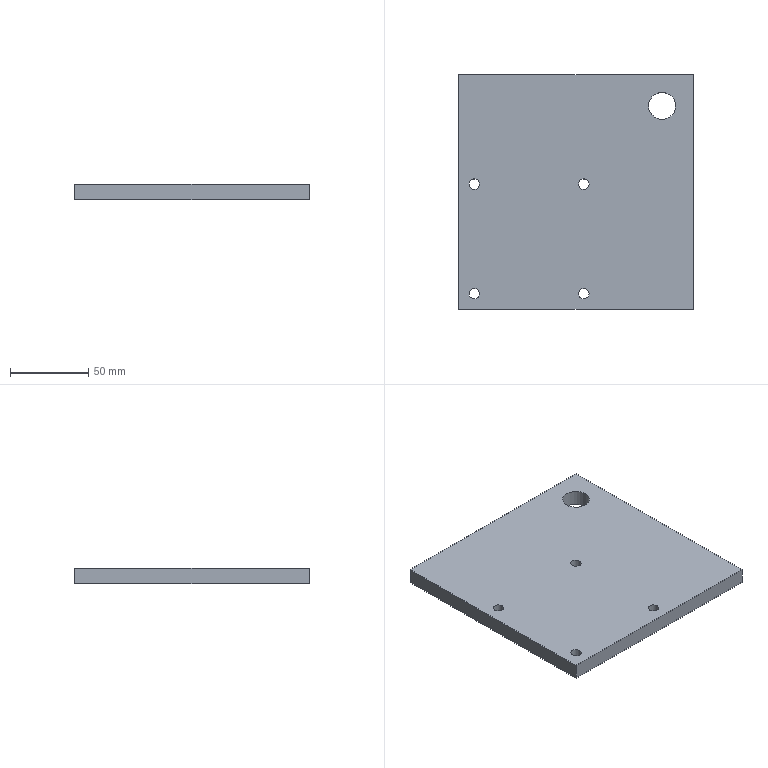Part | STEP file | SynoNew-0304-044 | 1 solid | 11 faces | box 150 x 150 x 10 mm | volume 221263 mm3 | plane 6 | cylinder 5 | commonest cylinder face diameters 6.647 x4 17.294 x1
STEP:
#1=CARTESIAN_POINT('',(-68.323,5.,0.));
#2=VERTEX_POINT('',#1);
#3=CARTESIAN_POINT('',(-61.676,5.,0.));
#4=VERTEX_POINT('',#3);
#5=CARTESIAN_POINT('',(-65.,5.,0.));
#6=DIRECTION('',(0.,0.,1.));
#7=DIRECTION('',(-1.,0.,0.));
#8=AXIS2_PLACEMENT_3D('',#5,#6,#7);
#9=CIRCLE('',#8,3.324);
#10=EDGE_CURVE('',#2,#4,#9,.T.);
#11=ORIENTED_EDGE('',*,*,#10,.F.);
#12=CARTESIAN_POINT('',(-65.,5.,0.));
#13=DIRECTION('',(0.,0.,1.));
#14=DIRECTION('',(-1.,0.,0.));
#15=AXIS2_PLACEMENT_3D('',#12,#13,#14);
#16=CIRCLE('',#15,3.324);
#17=EDGE_CURVE('',#4,#2,#16,.T.);
#18=ORIENTED_EDGE('',*,*,#17,.F.);
#19=CARTESIAN_POINT('',(-61.676,5.,10.));
#20=VERTEX_POINT('',#19);
#21=CARTESIAN_POINT('',(-61.676,5.,212.368));
#22=DIRECTION('',(0.,0.,1.));
#23=VECTOR('',#22,3.324);
#24=LINE('',#21,#23);
#25=EDGE_CURVE('',#4,#20,#24,.T.);
#26=ORIENTED_EDGE('',*,*,#25,.T.);
#27=CARTESIAN_POINT('',(-65.,5.,10.));
#28=DIRECTION('',(0.,0.,-1.));
#29=DIRECTION('',(-1.,0.,0.));
#30=AXIS2_PLACEMENT_3D('',#27,#28,#29);
#31=CIRCLE('',#30,3.324);
#32=EDGE_CURVE('',#20,#20,#31,.T.);
#33=ORIENTED_EDGE('',*,*,#32,.F.);
#34=ORIENTED_EDGE('',*,*,#25,.F.);
#35=EDGE_LOOP('',(#11,#18,#26,#33,#34));
#36=FACE_OUTER_BOUND('',#35,.T.);
#37=CARTESIAN_POINT('',(-65.,5.,212.368));
#38=DIRECTION('',(0.,0.,-1.));
#39=DIRECTION('',(-1.,0.,0.));
#40=AXIS2_PLACEMENT_3D('',#37,#38,#39);
#41=CYLINDRICAL_SURFACE('',#40,3.324);
#42=ADVANCED_FACE('',(#36),#41,.F.);
#43=CARTESIAN_POINT('',(1.677,-65.,0.));
#44=VERTEX_POINT('',#43);
#45=CARTESIAN_POINT('',(8.324,-65.,0.));
#46=VERTEX_POINT('',#45);
#47=CARTESIAN_POINT('',(5.,-65.,0.));
#48=DIRECTION('',(0.,0.,1.));
#49=DIRECTION('',(-1.,0.,0.));
#50=AXIS2_PLACEMENT_3D('',#47,#48,#49);
#51=CIRCLE('',#50,3.324);
#52=EDGE_CURVE('',#44,#46,#51,.T.);
#53=ORIENTED_EDGE('',*,*,#52,.F.);
#54=CARTESIAN_POINT('',(5.,-65.,0.));
#55=DIRECTION('',(0.,0.,1.));
#56=DIRECTION('',(-1.,0.,0.));
#57=AXIS2_PLACEMENT_3D('',#54,#55,#56);
#58=CIRCLE('',#57,3.324);
#59=EDGE_CURVE('',#46,#44,#58,.T.);
#60=ORIENTED_EDGE('',*,*,#59,.F.);
#61=CARTESIAN_POINT('',(8.324,-65.,10.));
#62=VERTEX_POINT('',#61);
#63=CARTESIAN_POINT('',(8.324,-65.,212.368));
#64=DIRECTION('',(0.,0.,1.));
#65=VECTOR('',#64,3.324);
#66=LINE('',#63,#65);
#67=EDGE_CURVE('',#46,#62,#66,.T.);
#68=ORIENTED_EDGE('',*,*,#67,.T.);
#69=CARTESIAN_POINT('',(5.,-65.,10.));
#70=DIRECTION('',(0.,0.,-1.));
#71=DIRECTION('',(-1.,0.,0.));
#72=AXIS2_PLACEMENT_3D('',#69,#70,#71);
#73=CIRCLE('',#72,3.324);
#74=EDGE_CURVE('',#62,#62,#73,.T.);
#75=ORIENTED_EDGE('',*,*,#74,.F.);
#76=ORIENTED_EDGE('',*,*,#67,.F.);
#77=EDGE_LOOP('',(#53,#60,#68,#75,#76));
#78=FACE_OUTER_BOUND('',#77,.T.);
#79=CARTESIAN_POINT('',(5.,-65.,212.368));
#80=DIRECTION('',(0.,0.,-1.));
#81=DIRECTION('',(-1.,0.,0.));
#82=AXIS2_PLACEMENT_3D('',#79,#80,#81);
#83=CYLINDRICAL_SURFACE('',#82,3.324);
#84=ADVANCED_FACE('',(#78),#83,.F.);
#85=CARTESIAN_POINT('',(1.677,5.,0.));
#86=VERTEX_POINT('',#85);
#87=CARTESIAN_POINT('',(8.324,5.,0.));
#88=VERTEX_POINT('',#87);
#89=CARTESIAN_POINT('',(5.,5.,0.));
#90=DIRECTION('',(0.,0.,1.));
#91=DIRECTION('',(-1.,0.,0.));
#92=AXIS2_PLACEMENT_3D('',#89,#90,#91);
#93=CIRCLE('',#92,3.324);
#94=EDGE_CURVE('',#86,#88,#93,.T.);
#95=ORIENTED_EDGE('',*,*,#94,.F.);
#96=CARTESIAN_POINT('',(5.,5.,0.));
#97=DIRECTION('',(0.,0.,1.));
#98=DIRECTION('',(-1.,0.,0.));
#99=AXIS2_PLACEMENT_3D('',#96,#97,#98);
#100=CIRCLE('',#99,3.324);
#101=EDGE_CURVE('',#88,#86,#100,.T.);
#102=ORIENTED_EDGE('',*,*,#101,.F.);
#103=CARTESIAN_POINT('',(8.324,5.,10.));
#104=VERTEX_POINT('',#103);
#105=CARTESIAN_POINT('',(8.324,5.,212.368));
#106=DIRECTION('',(0.,0.,1.));
#107=VECTOR('',#106,3.324);
#108=LINE('',#105,#107);
#109=EDGE_CURVE('',#88,#104,#108,.T.);
#110=ORIENTED_EDGE('',*,*,#109,.T.);
#111=CARTESIAN_POINT('',(5.,5.,10.));
#112=DIRECTION('',(0.,0.,-1.));
#113=DIRECTION('',(-1.,0.,0.));
#114=AXIS2_PLACEMENT_3D('',#111,#112,#113);
#115=CIRCLE('',#114,3.324);
#116=EDGE_CURVE('',#104,#104,#115,.T.);
#117=ORIENTED_EDGE('',*,*,#116,.F.);
#118=ORIENTED_EDGE('',*,*,#109,.F.);
#119=EDGE_LOOP('',(#95,#102,#110,#117,#118));
#120=FACE_OUTER_BOUND('',#119,.T.);
#121=CARTESIAN_POINT('',(5.,5.,212.368));
#122=DIRECTION('',(0.,0.,-1.));
#123=DIRECTION('',(-1.,0.,0.));
#124=AXIS2_PLACEMENT_3D('',#121,#122,#123);
#125=CYLINDRICAL_SURFACE('',#124,3.324);
#126=ADVANCED_FACE('',(#120),#125,.F.);
#127=CARTESIAN_POINT('',(-68.323,-65.,0.));
#128=VERTEX_POINT('',#127);
#129=CARTESIAN_POINT('',(-61.676,-65.,0.));
#130=VERTEX_POINT('',#129);
#131=CARTESIAN_POINT('',(-65.,-65.,0.));
#132=DIRECTION('',(0.,0.,1.));
#133=DIRECTION('',(-1.,0.,0.));
#134=AXIS2_PLACEMENT_3D('',#131,#132,#133);
#135=CIRCLE('',#134,3.324);
#136=EDGE_CURVE('',#128,#130,#135,.T.);
#137=ORIENTED_EDGE('',*,*,#136,.F.);
#138=CARTESIAN_POINT('',(-65.,-65.,0.));
#139=DIRECTION('',(0.,0.,1.));
#140=DIRECTION('',(-1.,0.,0.));
#141=AXIS2_PLACEMENT_3D('',#138,#139,#140);
#142=CIRCLE('',#141,3.324);
#143=EDGE_CURVE('',#130,#128,#142,.T.);
#144=ORIENTED_EDGE('',*,*,#143,.F.);
#145=CARTESIAN_POINT('',(-61.676,-65.,10.));
#146=VERTEX_POINT('',#145);
#147=CARTESIAN_POINT('',(-61.676,-65.,212.368));
#148=DIRECTION('',(0.,0.,1.));
#149=VECTOR('',#148,3.324);
#150=LINE('',#147,#149);
#151=EDGE_CURVE('',#130,#146,#150,.T.);
#152=ORIENTED_EDGE('',*,*,#151,.T.);
#153=CARTESIAN_POINT('',(-65.,-65.,10.));
#154=DIRECTION('',(0.,0.,-1.));
#155=DIRECTION('',(-1.,0.,0.));
#156=AXIS2_PLACEMENT_3D('',#153,#154,#155);
#157=CIRCLE('',#156,3.324);
#158=EDGE_CURVE('',#146,#146,#157,.T.);
#159=ORIENTED_EDGE('',*,*,#158,.F.);
#160=ORIENTED_EDGE('',*,*,#151,.F.);
#161=EDGE_LOOP('',(#137,#144,#152,#159,#160));
#162=FACE_OUTER_BOUND('',#161,.T.);
#163=CARTESIAN_POINT('',(-65.,-65.,212.368));
#164=DIRECTION('',(0.,0.,-1.));
#165=DIRECTION('',(-1.,0.,0.));
#166=AXIS2_PLACEMENT_3D('',#163,#164,#165);
#167=CYLINDRICAL_SURFACE('',#166,3.324);
#168=ADVANCED_FACE('',(#162),#167,.F.);
#169=CARTESIAN_POINT('',(63.647,55.,10.));
#170=VERTEX_POINT('',#169);
#171=CARTESIAN_POINT('',(46.353,55.,10.));
#172=VERTEX_POINT('',#171);
#173=CARTESIAN_POINT('',(55.,55.,10.));
#174=DIRECTION('',(0.,0.,-1.));
#175=DIRECTION('',(1.,0.,0.));
#176=AXIS2_PLACEMENT_3D('',#173,#174,#175);
#177=CIRCLE('',#176,8.647);
#178=EDGE_CURVE('',#170,#172,#177,.T.);
#179=ORIENTED_EDGE('',*,*,#178,.F.);
#180=CARTESIAN_POINT('',(55.,55.,10.));
#181=DIRECTION('',(0.,0.,-1.));
#182=DIRECTION('',(1.,0.,0.));
#183=AXIS2_PLACEMENT_3D('',#180,#181,#182);
#184=CIRCLE('',#183,8.647);
#185=EDGE_CURVE('',#172,#170,#184,.T.);
#186=ORIENTED_EDGE('',*,*,#185,.F.);
#187=CARTESIAN_POINT('',(46.353,55.,0.));
#188=VERTEX_POINT('',#187);
#189=CARTESIAN_POINT('',(46.353,55.,-202.368));
#190=DIRECTION('',(0.,0.,-1.));
#191=VECTOR('',#190,8.647);
#192=LINE('',#189,#191);
#193=EDGE_CURVE('',#172,#188,#192,.T.);
#194=ORIENTED_EDGE('',*,*,#193,.T.);
#195=CARTESIAN_POINT('',(55.,55.,0.));
#196=DIRECTION('',(0.,0.,1.));
#197=DIRECTION('',(1.,0.,0.));
#198=AXIS2_PLACEMENT_3D('',#195,#196,#197);
#199=CIRCLE('',#198,8.647);
#200=EDGE_CURVE('',#188,#188,#199,.T.);
#201=ORIENTED_EDGE('',*,*,#200,.F.);
#202=ORIENTED_EDGE('',*,*,#193,.F.);
#203=EDGE_LOOP('',(#179,#186,#194,#201,#202));
#204=FACE_OUTER_BOUND('',#203,.T.);
#205=CARTESIAN_POINT('',(55.,55.,-202.368));
#206=DIRECTION('',(0.,0.,1.));
#207=DIRECTION('',(1.,0.,0.));
#208=AXIS2_PLACEMENT_3D('',#205,#206,#207);
#209=CYLINDRICAL_SURFACE('',#208,8.647);
#210=ADVANCED_FACE('',(#204),#209,.F.);
#211=CARTESIAN_POINT('',(-75.,-75.,0.));
#212=VERTEX_POINT('',#211);
#213=CARTESIAN_POINT('',(75.,-75.,0.));
#214=VERTEX_POINT('',#213);
#215=CARTESIAN_POINT('',(-75.,-75.,0.));
#216=DIRECTION('',(1.,0.,0.));
#217=VECTOR('',#216,10.);
#218=LINE('',#215,#217);
#219=EDGE_CURVE('',#212,#214,#218,.T.);
#220=ORIENTED_EDGE('',*,*,#219,.T.);
#221=CARTESIAN_POINT('',(75.,-75.,10.));
#222=VERTEX_POINT('',#221);
#223=CARTESIAN_POINT('',(75.,-75.,0.));
#224=DIRECTION('',(0.,0.,1.));
#225=VECTOR('',#224,10.);
#226=LINE('',#223,#225);
#227=EDGE_CURVE('',#214,#222,#226,.T.);
#228=ORIENTED_EDGE('',*,*,#227,.T.);
#229=CARTESIAN_POINT('',(-75.,-75.,10.));
#230=VERTEX_POINT('',#229);
#231=CARTESIAN_POINT('',(-75.,-75.,10.));
#232=DIRECTION('',(1.,0.,0.));
#233=VECTOR('',#232,10.);
#234=LINE('',#231,#233);
#235=EDGE_CURVE('',#230,#222,#234,.T.);
#236=ORIENTED_EDGE('',*,*,#235,.F.);
#237=CARTESIAN_POINT('',(-75.,-75.,0.));
#238=DIRECTION('',(0.,0.,1.));
#239=VECTOR('',#238,10.);
#240=LINE('',#237,#239);
#241=EDGE_CURVE('',#212,#230,#240,.T.);
#242=ORIENTED_EDGE('',*,*,#241,.F.);
#243=EDGE_LOOP('',(#220,#228,#236,#242));
#244=FACE_OUTER_BOUND('',#243,.T.);
#245=CARTESIAN_POINT('',(-75.,-75.,0.));
#246=DIRECTION('',(0.,-1.,0.));
#247=DIRECTION('',(1.,0.,0.));
#248=AXIS2_PLACEMENT_3D('',#245,#246,#247);
#249=PLANE('',#248);
#250=ADVANCED_FACE('',(#244),#249,.T.);
#251=CARTESIAN_POINT('',(-75.,75.,0.));
#252=VERTEX_POINT('',#251);
#253=CARTESIAN_POINT('',(-75.,75.,0.));
#254=DIRECTION('',(0.,-1.,0.));
#255=VECTOR('',#254,10.);
#256=LINE('',#253,#255);
#257=EDGE_CURVE('',#252,#212,#256,.T.);
#258=ORIENTED_EDGE('',*,*,#257,.T.);
#259=ORIENTED_EDGE('',*,*,#241,.T.);
#260=CARTESIAN_POINT('',(-75.,75.,10.));
#261=VERTEX_POINT('',#260);
#262=CARTESIAN_POINT('',(-75.,75.,10.));
#263=DIRECTION('',(0.,-1.,0.));
#264=VECTOR('',#263,10.);
#265=LINE('',#262,#264);
#266=EDGE_CURVE('',#261,#230,#265,.T.);
#267=ORIENTED_EDGE('',*,*,#266,.F.);
#268=CARTESIAN_POINT('',(-75.,75.,0.));
#269=DIRECTION('',(0.,0.,1.));
#270=VECTOR('',#269,10.);
#271=LINE('',#268,#270);
#272=EDGE_CURVE('',#252,#261,#271,.T.);
#273=ORIENTED_EDGE('',*,*,#272,.F.);
#274=EDGE_LOOP('',(#258,#259,#267,#273));
#275=FACE_OUTER_BOUND('',#274,.T.);
#276=CARTESIAN_POINT('',(-75.,75.,0.));
#277=DIRECTION('',(-1.,0.,0.));
#278=DIRECTION('',(0.,-1.,0.));
#279=AXIS2_PLACEMENT_3D('',#276,#277,#278);
#280=PLANE('',#279);
#281=ADVANCED_FACE('',(#275),#280,.T.);
#282=CARTESIAN_POINT('',(75.,75.,0.));
#283=VERTEX_POINT('',#282);
#284=CARTESIAN_POINT('',(75.,75.,0.));
#285=DIRECTION('',(-1.,0.,0.));
#286=VECTOR('',#285,10.);
#287=LINE('',#284,#286);
#288=EDGE_CURVE('',#283,#252,#287,.T.);
#289=ORIENTED_EDGE('',*,*,#288,.T.);
#290=ORIENTED_EDGE('',*,*,#272,.T.);
#291=CARTESIAN_POINT('',(75.,75.,10.));
#292=VERTEX_POINT('',#291);
#293=CARTESIAN_POINT('',(75.,75.,10.));
#294=DIRECTION('',(-1.,0.,0.));
#295=VECTOR('',#294,10.);
#296=LINE('',#293,#295);
#297=EDGE_CURVE('',#292,#261,#296,.T.);
#298=ORIENTED_EDGE('',*,*,#297,.F.);
#299=CARTESIAN_POINT('',(75.,75.,0.));
#300=DIRECTION('',(0.,0.,1.));
#301=VECTOR('',#300,10.);
#302=LINE('',#299,#301);
#303=EDGE_CURVE('',#283,#292,#302,.T.);
#304=ORIENTED_EDGE('',*,*,#303,.F.);
#305=EDGE_LOOP('',(#289,#290,#298,#304));
#306=FACE_OUTER_BOUND('',#305,.T.);
#307=CARTESIAN_POINT('',(75.,75.,0.));
#308=DIRECTION('',(0.,1.,0.));
#309=DIRECTION('',(-1.,0.,0.));
#310=AXIS2_PLACEMENT_3D('',#307,#308,#309);
#311=PLANE('',#310);
#312=ADVANCED_FACE('',(#306),#311,.T.);
#313=CARTESIAN_POINT('',(75.,-75.,0.));
#314=DIRECTION('',(0.,1.,0.));
#315=VECTOR('',#314,10.);
#316=LINE('',#313,#315);
#317=EDGE_CURVE('',#214,#283,#316,.T.);
#318=ORIENTED_EDGE('',*,*,#317,.T.);
#319=ORIENTED_EDGE('',*,*,#303,.T.);
#320=CARTESIAN_POINT('',(75.,-75.,10.));
#321=DIRECTION('',(0.,1.,0.));
#322=VECTOR('',#321,10.);
#323=LINE('',#320,#322);
#324=EDGE_CURVE('',#222,#292,#323,.T.);
#325=ORIENTED_EDGE('',*,*,#324,.F.);
#326=ORIENTED_EDGE('',*,*,#227,.F.);
#327=EDGE_LOOP('',(#318,#319,#325,#326));
#328=FACE_OUTER_BOUND('',#327,.T.);
#329=CARTESIAN_POINT('',(75.,-75.,0.));
#330=DIRECTION('',(1.,0.,0.));
#331=DIRECTION('',(0.,1.,0.));
#332=AXIS2_PLACEMENT_3D('',#329,#330,#331);
#333=PLANE('',#332);
#334=ADVANCED_FACE('',(#328),#333,.T.);
#335=ORIENTED_EDGE('',*,*,#324,.T.);
#336=ORIENTED_EDGE('',*,*,#297,.T.);
#337=ORIENTED_EDGE('',*,*,#266,.T.);
#338=ORIENTED_EDGE('',*,*,#235,.T.);
#339=EDGE_LOOP('',(#335,#336,#337,#338));
#340=FACE_OUTER_BOUND('',#339,.T.);
#341=ORIENTED_EDGE('',*,*,#32,.T.);
#342=EDGE_LOOP('',(#341));
#343=FACE_BOUND('',#342,.T.);
#344=ORIENTED_EDGE('',*,*,#74,.T.);
#345=EDGE_LOOP('',(#344));
#346=FACE_BOUND('',#345,.T.);
#347=ORIENTED_EDGE('',*,*,#116,.T.);
#348=EDGE_LOOP('',(#347));
#349=FACE_BOUND('',#348,.T.);
#350=ORIENTED_EDGE('',*,*,#158,.T.);
#351=EDGE_LOOP('',(#350));
#352=FACE_BOUND('',#351,.T.);
#353=ORIENTED_EDGE('',*,*,#178,.T.);
#354=ORIENTED_EDGE('',*,*,#185,.T.);
#355=EDGE_LOOP('',(#353,#354));
#356=FACE_BOUND('',#355,.T.);
#357=CARTESIAN_POINT('',(0.,0.,10.));
#358=DIRECTION('',(0.,0.,1.));
#359=DIRECTION('',(1.,0.,0.));
#360=AXIS2_PLACEMENT_3D('',#357,#358,#359);
#361=PLANE('',#360);
#362=ADVANCED_FACE('',(#340,#343,#346,#349,#352,#356),#361,.T.);
#363=ORIENTED_EDGE('',*,*,#317,.F.);
#364=ORIENTED_EDGE('',*,*,#219,.F.);
#365=ORIENTED_EDGE('',*,*,#257,.F.);
#366=ORIENTED_EDGE('',*,*,#288,.F.);
#367=EDGE_LOOP('',(#363,#364,#365,#366));
#368=FACE_OUTER_BOUND('',#367,.T.);
#369=ORIENTED_EDGE('',*,*,#10,.T.);
#370=ORIENTED_EDGE('',*,*,#17,.T.);
#371=EDGE_LOOP('',(#369,#370));
#372=FACE_BOUND('',#371,.T.);
#373=ORIENTED_EDGE('',*,*,#52,.T.);
#374=ORIENTED_EDGE('',*,*,#59,.T.);
#375=EDGE_LOOP('',(#373,#374));
#376=FACE_BOUND('',#375,.T.);
#377=ORIENTED_EDGE('',*,*,#94,.T.);
#378=ORIENTED_EDGE('',*,*,#101,.T.);
#379=EDGE_LOOP('',(#377,#378));
#380=FACE_BOUND('',#379,.T.);
#381=ORIENTED_EDGE('',*,*,#136,.T.);
#382=ORIENTED_EDGE('',*,*,#143,.T.);
#383=EDGE_LOOP('',(#381,#382));
#384=FACE_BOUND('',#383,.T.);
#385=ORIENTED_EDGE('',*,*,#200,.T.);
#386=EDGE_LOOP('',(#385));
#387=FACE_BOUND('',#386,.T.);
#388=CARTESIAN_POINT('',(0.,0.,0.));
#389=DIRECTION('',(0.,0.,1.));
#390=DIRECTION('',(1.,0.,0.));
#391=AXIS2_PLACEMENT_3D('',#388,#389,#390);
#392=PLANE('',#391);
#393=ADVANCED_FACE('',(#368,#372,#376,#380,#384,#387),#392,.F.);
#394=CLOSED_SHELL('',(#42,#84,#126,#168,#210,#250,#281,#312,#334,#362,#393));
#395=MANIFOLD_SOLID_BREP('',#394);
#396=(LENGTH_UNIT()NAMED_UNIT(*)SI_UNIT(.MILLI.,.METRE.));
#397=UNCERTAINTY_MEASURE_WITH_UNIT(LENGTH_MEASURE(0.01),#396,'','');
#398=(NAMED_UNIT(*)PLANE_ANGLE_UNIT()SI_UNIT($,.RADIAN.));
#399=(NAMED_UNIT(*)SI_UNIT($,.STERADIAN.)SOLID_ANGLE_UNIT());
#400=(GEOMETRIC_REPRESENTATION_CONTEXT(3)GLOBAL_UNCERTAINTY_ASSIGNED_CONTEXT((#397))GLOBAL_UNIT_ASSIGNED_CONTEXT((#396,#398,#399))REPRESENTATION_CONTEXT('',''));
#401=ADVANCED_BREP_SHAPE_REPRESENTATION('',(#395),#400);